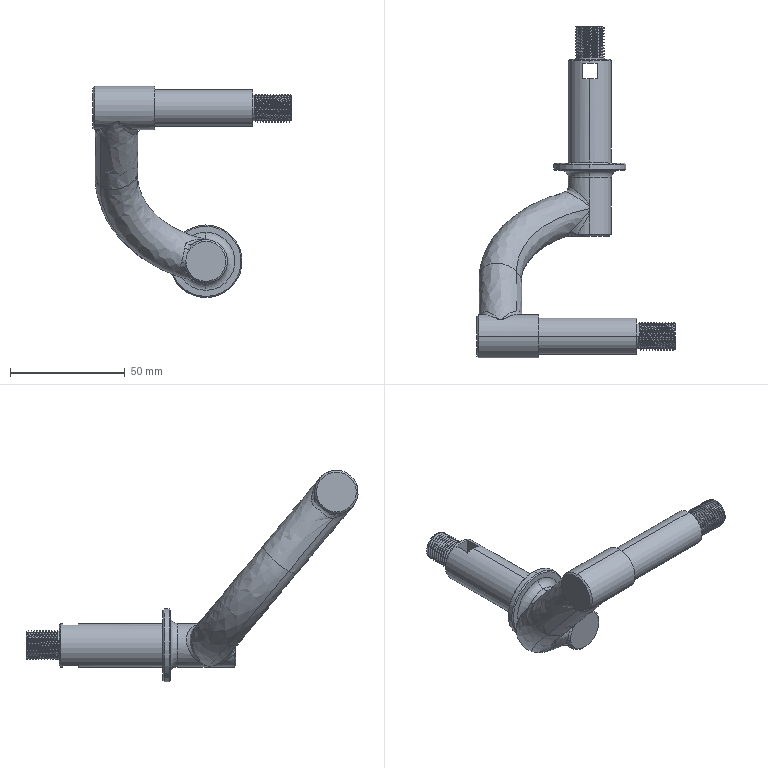Part | SolidWorks | features ICE 7, Chamfer 5, Fillet 3, SweepThread 2, Extrusion 1, Revolution 1, Sweep 1 | 1 solid | 126 faces | box 86.354 x 144.501 x 91.948 mm | volume 66693 mm3 | cylinder 65 | plane 22 | spline 21 | cone 16 | torus 2 | commonest cylinder face diameters 12.243 x25 12.7 x22 18.923 x7 1.587 x4 11.112 x3 15.875 x2